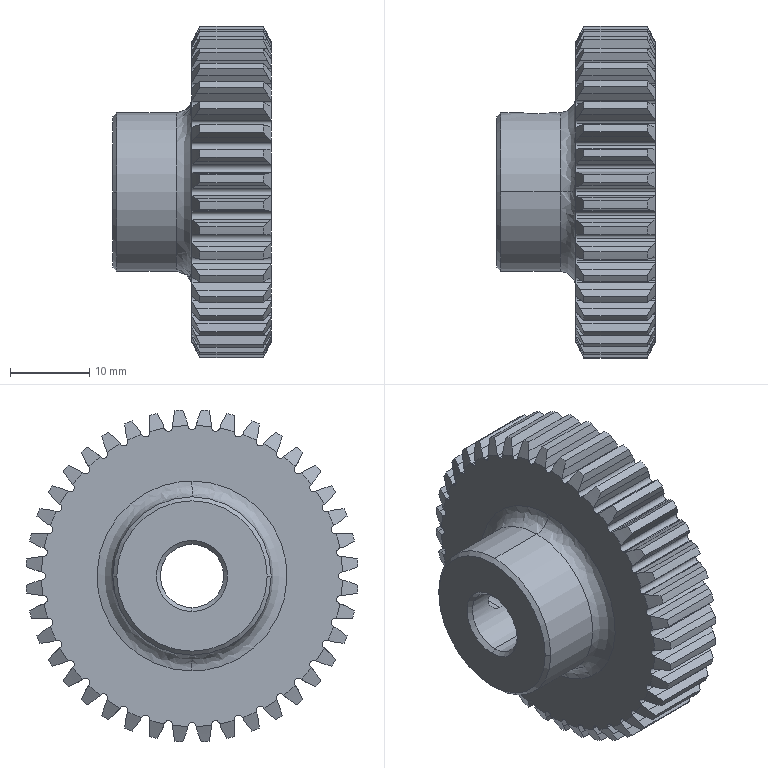Part | STEP file | 06-09 1-40 gear | 1 solid | 354 faces | box 20 x 41.938 x 41.938 mm | volume 14422 mm3 | plane 163 | cylinder 103 | cone 86 | spline 2 | commonest cylinder face diameters 1 x57 42 x40 3.3 x2 8 x2 20 x2